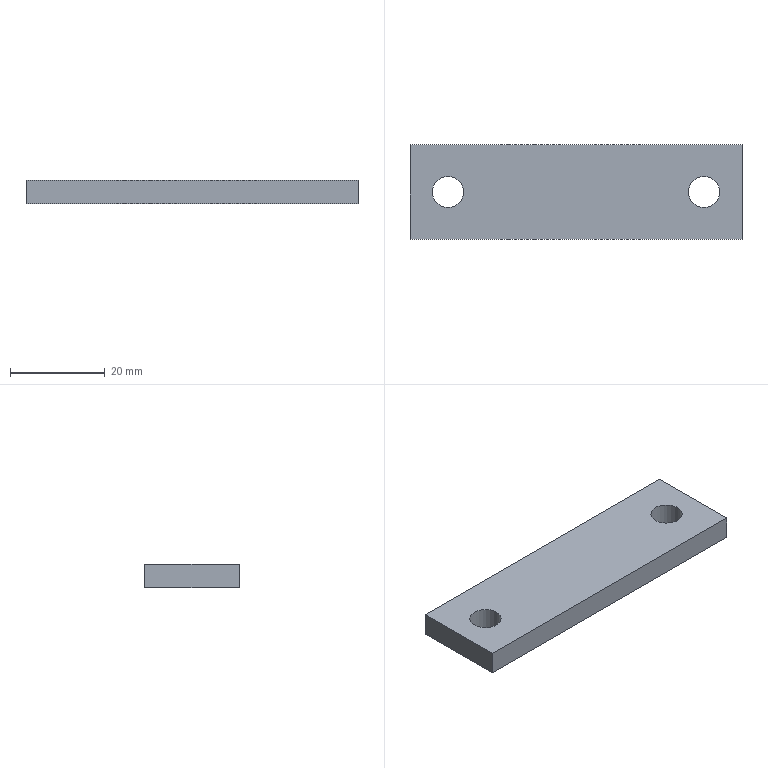Part | NX | 1 solid | 8 faces | box 70 x 20 x 5 mm | volume 6658 mm3 | plane 6 | cylinder 2 | commonest cylinder face diameters 6.6 x2
STEP:
#1=CARTESIAN_POINT('',(35.,-10.,0.));
#2=VERTEX_POINT('',#1);
#3=CARTESIAN_POINT('',(35.,10.,0.));
#4=VERTEX_POINT('',#3);
#5=CARTESIAN_POINT('',(35.,-10.,0.));
#6=DIRECTION('',(0.,1.,0.));
#7=VECTOR('',#6,1000.);
#8=LINE('',#5,#7);
#9=EDGE_CURVE('',#2,#4,#8,.T.);
#10=ORIENTED_EDGE('',*,*,#9,.T.);
#11=CARTESIAN_POINT('',(35.,10.,5.));
#12=VERTEX_POINT('',#11);
#13=CARTESIAN_POINT('',(35.,10.,5.));
#14=DIRECTION('',(0.,0.,-1.));
#15=VECTOR('',#14,1000.);
#16=LINE('',#13,#15);
#17=EDGE_CURVE('',#12,#4,#16,.T.);
#18=ORIENTED_EDGE('',*,*,#17,.F.);
#19=CARTESIAN_POINT('',(35.,-10.,5.));
#20=VERTEX_POINT('',#19);
#21=CARTESIAN_POINT('',(35.,-10.,5.));
#22=DIRECTION('',(0.,1.,0.));
#23=VECTOR('',#22,1000.);
#24=LINE('',#21,#23);
#25=EDGE_CURVE('',#20,#12,#24,.T.);
#26=ORIENTED_EDGE('',*,*,#25,.F.);
#27=CARTESIAN_POINT('',(35.,-10.,5.));
#28=DIRECTION('',(0.,0.,-1.));
#29=VECTOR('',#28,1000.);
#30=LINE('',#27,#29);
#31=EDGE_CURVE('',#20,#2,#30,.T.);
#32=ORIENTED_EDGE('',*,*,#31,.T.);
#33=EDGE_LOOP('',(#10,#18,#26,#32));
#34=FACE_BOUND('',#33,.T.);
#35=CARTESIAN_POINT('',(35.,-10.,5.));
#36=DIRECTION('',(-1.,0.,0.));
#37=DIRECTION('',(0.,0.,1.));
#38=AXIS2_PLACEMENT_3D('',#35,#36,#37);
#39=PLANE('',#38);
#40=ADVANCED_FACE('',(#34),#39,.F.);
#41=CARTESIAN_POINT('',(-35.,10.,0.));
#42=VERTEX_POINT('',#41);
#43=CARTESIAN_POINT('',(-35.,10.,0.));
#44=DIRECTION('',(-1.,0.,0.));
#45=VECTOR('',#44,1000.);
#46=LINE('',#43,#45);
#47=EDGE_CURVE('',#4,#42,#46,.T.);
#48=ORIENTED_EDGE('',*,*,#47,.T.);
#49=CARTESIAN_POINT('',(-35.,10.,5.));
#50=VERTEX_POINT('',#49);
#51=CARTESIAN_POINT('',(-35.,10.,5.));
#52=DIRECTION('',(0.,0.,-1.));
#53=VECTOR('',#52,1000.);
#54=LINE('',#51,#53);
#55=EDGE_CURVE('',#50,#42,#54,.T.);
#56=ORIENTED_EDGE('',*,*,#55,.F.);
#57=CARTESIAN_POINT('',(-35.,10.,5.));
#58=DIRECTION('',(-1.,0.,0.));
#59=VECTOR('',#58,1000.);
#60=LINE('',#57,#59);
#61=EDGE_CURVE('',#12,#50,#60,.T.);
#62=ORIENTED_EDGE('',*,*,#61,.F.);
#63=ORIENTED_EDGE('',*,*,#17,.T.);
#64=EDGE_LOOP('',(#48,#56,#62,#63));
#65=FACE_BOUND('',#64,.T.);
#66=CARTESIAN_POINT('',(-35.,10.,5.));
#67=DIRECTION('',(0.,-1.,0.));
#68=DIRECTION('',(0.,0.,-1.));
#69=AXIS2_PLACEMENT_3D('',#66,#67,#68);
#70=PLANE('',#69);
#71=ADVANCED_FACE('',(#65),#70,.F.);
#72=CARTESIAN_POINT('',(-35.,-10.,0.));
#73=VERTEX_POINT('',#72);
#74=CARTESIAN_POINT('',(-35.,-10.,0.));
#75=DIRECTION('',(0.,-1.,0.));
#76=VECTOR('',#75,1000.);
#77=LINE('',#74,#76);
#78=EDGE_CURVE('',#42,#73,#77,.T.);
#79=ORIENTED_EDGE('',*,*,#78,.T.);
#80=CARTESIAN_POINT('',(-35.,-10.,5.));
#81=VERTEX_POINT('',#80);
#82=CARTESIAN_POINT('',(-35.,-10.,5.));
#83=DIRECTION('',(0.,0.,-1.));
#84=VECTOR('',#83,1000.);
#85=LINE('',#82,#84);
#86=EDGE_CURVE('',#81,#73,#85,.T.);
#87=ORIENTED_EDGE('',*,*,#86,.F.);
#88=CARTESIAN_POINT('',(-35.,-10.,5.));
#89=DIRECTION('',(0.,-1.,0.));
#90=VECTOR('',#89,1000.);
#91=LINE('',#88,#90);
#92=EDGE_CURVE('',#50,#81,#91,.T.);
#93=ORIENTED_EDGE('',*,*,#92,.F.);
#94=ORIENTED_EDGE('',*,*,#55,.T.);
#95=EDGE_LOOP('',(#79,#87,#93,#94));
#96=FACE_BOUND('',#95,.T.);
#97=CARTESIAN_POINT('',(-35.,-10.,5.));
#98=DIRECTION('',(1.,0.,0.));
#99=DIRECTION('',(0.,0.,-1.));
#100=AXIS2_PLACEMENT_3D('',#97,#98,#99);
#101=PLANE('',#100);
#102=ADVANCED_FACE('',(#96),#101,.F.);
#103=CARTESIAN_POINT('',(-35.,-10.,0.));
#104=DIRECTION('',(1.,0.,0.));
#105=VECTOR('',#104,1000.);
#106=LINE('',#103,#105);
#107=EDGE_CURVE('',#73,#2,#106,.T.);
#108=ORIENTED_EDGE('',*,*,#107,.T.);
#109=ORIENTED_EDGE('',*,*,#31,.F.);
#110=CARTESIAN_POINT('',(-35.,-10.,5.));
#111=DIRECTION('',(1.,0.,0.));
#112=VECTOR('',#111,1000.);
#113=LINE('',#110,#112);
#114=EDGE_CURVE('',#81,#20,#113,.T.);
#115=ORIENTED_EDGE('',*,*,#114,.F.);
#116=ORIENTED_EDGE('',*,*,#86,.T.);
#117=EDGE_LOOP('',(#108,#109,#115,#116));
#118=FACE_BOUND('',#117,.T.);
#119=CARTESIAN_POINT('',(-35.,-10.,5.));
#120=DIRECTION('',(0.,1.,0.));
#121=DIRECTION('',(0.,0.,1.));
#122=AXIS2_PLACEMENT_3D('',#119,#120,#121);
#123=PLANE('',#122);
#124=ADVANCED_FACE('',(#118),#123,.F.);
#125=CARTESIAN_POINT('',(-23.7,0.,5.));
#126=VERTEX_POINT('',#125);
#127=CARTESIAN_POINT('',(-27.,0.,5.));
#128=DIRECTION('',(0.,0.,1.));
#129=DIRECTION('',(1.,0.,0.));
#130=AXIS2_PLACEMENT_3D('',#127,#128,#129);
#131=CIRCLE('',#130,3.3);
#132=EDGE_CURVE('',#126,#126,#131,.T.);
#133=ORIENTED_EDGE('',*,*,#132,.F.);
#134=EDGE_LOOP('',(#133));
#135=FACE_BOUND('',#134,.T.);
#136=CARTESIAN_POINT('',(30.3,0.,5.));
#137=VERTEX_POINT('',#136);
#138=CARTESIAN_POINT('',(27.,0.,5.));
#139=DIRECTION('',(0.,0.,1.));
#140=DIRECTION('',(1.,0.,0.));
#141=AXIS2_PLACEMENT_3D('',#138,#139,#140);
#142=CIRCLE('',#141,3.3);
#143=EDGE_CURVE('',#137,#137,#142,.T.);
#144=ORIENTED_EDGE('',*,*,#143,.F.);
#145=EDGE_LOOP('',(#144));
#146=FACE_BOUND('',#145,.T.);
#147=ORIENTED_EDGE('',*,*,#25,.T.);
#148=ORIENTED_EDGE('',*,*,#61,.T.);
#149=ORIENTED_EDGE('',*,*,#92,.T.);
#150=ORIENTED_EDGE('',*,*,#114,.T.);
#151=EDGE_LOOP('',(#147,#148,#149,#150));
#152=FACE_BOUND('',#151,.T.);
#153=CARTESIAN_POINT('',(0.,0.,5.));
#154=DIRECTION('',(0.,0.,-1.));
#155=DIRECTION('',(-1.,0.,0.));
#156=AXIS2_PLACEMENT_3D('',#153,#154,#155);
#157=PLANE('',#156);
#158=ADVANCED_FACE('',(#135,#146,#152),#157,.F.);
#159=CARTESIAN_POINT('',(-23.7,0.,0.));
#160=VERTEX_POINT('',#159);
#161=CARTESIAN_POINT('',(-27.,0.,0.));
#162=DIRECTION('',(0.,0.,1.));
#163=DIRECTION('',(1.,0.,0.));
#164=AXIS2_PLACEMENT_3D('',#161,#162,#163);
#165=CIRCLE('',#164,3.3);
#166=EDGE_CURVE('',#160,#160,#165,.T.);
#167=ORIENTED_EDGE('',*,*,#166,.T.);
#168=EDGE_LOOP('',(#167));
#169=FACE_BOUND('',#168,.T.);
#170=CARTESIAN_POINT('',(30.3,0.,0.));
#171=VERTEX_POINT('',#170);
#172=CARTESIAN_POINT('',(27.,0.,0.));
#173=DIRECTION('',(0.,0.,1.));
#174=DIRECTION('',(1.,0.,0.));
#175=AXIS2_PLACEMENT_3D('',#172,#173,#174);
#176=CIRCLE('',#175,3.3);
#177=EDGE_CURVE('',#171,#171,#176,.T.);
#178=ORIENTED_EDGE('',*,*,#177,.T.);
#179=EDGE_LOOP('',(#178));
#180=FACE_BOUND('',#179,.T.);
#181=ORIENTED_EDGE('',*,*,#9,.F.);
#182=ORIENTED_EDGE('',*,*,#107,.F.);
#183=ORIENTED_EDGE('',*,*,#78,.F.);
#184=ORIENTED_EDGE('',*,*,#47,.F.);
#185=EDGE_LOOP('',(#181,#182,#183,#184));
#186=FACE_BOUND('',#185,.T.);
#187=CARTESIAN_POINT('',(0.,0.,0.));
#188=DIRECTION('',(0.,0.,-1.));
#189=DIRECTION('',(-1.,0.,0.));
#190=AXIS2_PLACEMENT_3D('',#187,#188,#189);
#191=PLANE('',#190);
#192=ADVANCED_FACE('',(#169,#180,#186),#191,.T.);
#193=ORIENTED_EDGE('',*,*,#177,.F.);
#194=EDGE_LOOP('',(#193));
#195=FACE_BOUND('',#194,.T.);
#196=ORIENTED_EDGE('',*,*,#143,.T.);
#197=EDGE_LOOP('',(#196));
#198=FACE_BOUND('',#197,.T.);
#199=CARTESIAN_POINT('',(27.,0.,5.));
#200=DIRECTION('',(0.,0.,1.));
#201=DIRECTION('',(1.,0.,0.));
#202=AXIS2_PLACEMENT_3D('',#199,#200,#201);
#203=CYLINDRICAL_SURFACE('',#202,3.3);
#204=ADVANCED_FACE('',(#195,#198),#203,.F.);
#205=ORIENTED_EDGE('',*,*,#166,.F.);
#206=EDGE_LOOP('',(#205));
#207=FACE_BOUND('',#206,.T.);
#208=ORIENTED_EDGE('',*,*,#132,.T.);
#209=EDGE_LOOP('',(#208));
#210=FACE_BOUND('',#209,.T.);
#211=CARTESIAN_POINT('',(-27.,0.,5.));
#212=DIRECTION('',(0.,0.,1.));
#213=DIRECTION('',(1.,0.,0.));
#214=AXIS2_PLACEMENT_3D('',#211,#212,#213);
#215=CYLINDRICAL_SURFACE('',#214,3.3);
#216=ADVANCED_FACE('',(#207,#210),#215,.F.);
#217=CLOSED_SHELL('',(#40,#71,#102,#124,#158,#192,#204,#216));
#218=MANIFOLD_SOLID_BREP('',#217);
#219=(LENGTH_UNIT()NAMED_UNIT(*)SI_UNIT(.MILLI.,.METRE.));
#220=UNCERTAINTY_MEASURE_WITH_UNIT(LENGTH_MEASURE(0.00001),#219,'','');
#221=(NAMED_UNIT(*)PLANE_ANGLE_UNIT()SI_UNIT($,.RADIAN.));
#222=(NAMED_UNIT(*)SI_UNIT($,.STERADIAN.)SOLID_ANGLE_UNIT());
#223=(GEOMETRIC_REPRESENTATION_CONTEXT(3)GLOBAL_UNCERTAINTY_ASSIGNED_CONTEXT((#220))GLOBAL_UNIT_ASSIGNED_CONTEXT((#219,#221,#222))REPRESENTATION_CONTEXT('',''));
#224=ADVANCED_BREP_SHAPE_REPRESENTATION('',(#218),#223);